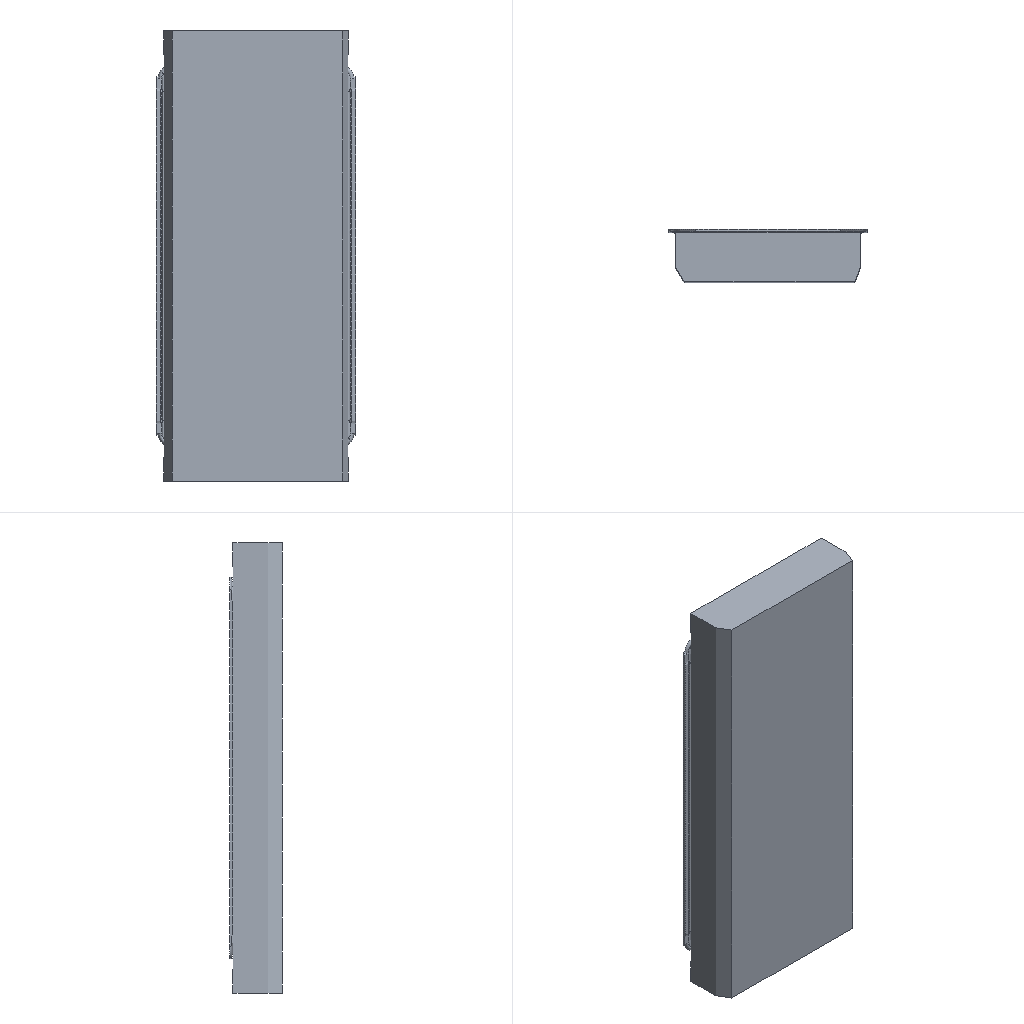Simulation study | ansys workbench
Set-up summary:
category,name,step,type,value,unit,region
solver,ansys_mapdl
solver,version,,,22.1
units,MPA,,stated
analysis,deck,,static,static
load_step,requested,,,1
analysis,nlgeom,,,False
mesh,nodes,,,345798
mesh,elements,,,249801
element_type,ANSYS 187 (type 1),,solid,1742
element_type,ANSYS 187 (type 2),,solid,204561
element_type,ANSYS 174 (type 3),,contact,7261
element_type,ANSYS 170 (type 4),,target,7261
element_type,ANSYS 154 (type 5),,surface,28976
load,load commands in deck,,count,1
bc,support commands in deck,,count,1
named_set,_FIXEDSU,,component
material,1,,in results
material,2,,in results
check,setup vs results,,match,28976 surface effect element(s) are not in the reader's mesh and were not compared
Ansys APDL input file, long lists of numbers shortened:
/batch
/config,noeldb,1     ! force off writing results to database
*get,_wallstrt,active,,time,wall
! ANSYS input file written by Workbench version 2022 R1
! File used for geometry attach: F:\ansys（分析文件汇总)\橡胶有限元分析\装配体简化.x_t
/title,wbnew--____ (B5)
! ****** Begin Custom Load Command Snippet ******
/COM, ACT Extensions:
/COM,     LSDYNA, 2021.1
/COM,
! ****** End   Custom Load Command Snippet ******
*DIM,_wb_ProjectScratch_dir,string,248
_wb_ProjectScratch_dir(1) = 'C:\Users\Administrator\AppData\Local\Temp\WB_Administrator_11288_2\_ProjectScratch\Scr4300\'
*DIM,_wb_SolverFiles_dir,string,248
_wb_SolverFiles_dir(1) = 'C:\Users\Administrator\AppData\Local\Temp\WB_Administrator_11288_2\wbnew_files\dp0\SYS\MECH\'
*DIM,_wb_userfiles_dir,string,248
_wb_userfiles_dir(1) = 'C:\Users\Administrator\AppData\Local\Temp\WB_Administrator_11288_2\wbnew_files\user_files\'
/com,--- Data in consistent NMM units. See Solving Units in the help system for more information.
/units,MPA
/nopr
/wb,file,start              !  signify a WB generated input file
/prep7
! Turn off shape checking because checks already performed inside WB mesher.
! See help system for more information.
SHPP,OFF,,NOWARN
/nolist
etcon,set             ! allow ANSYS to choose best KEYOP's for 180x elements, resets any applicable keyopt to MAPDL defaults
/com,*********** Nodes for the whole assembly ***********
nblock,3,,380377
(1i9,3e20.9e3)
        1    -7.883517716E+02    -5.000000000E+01    -1.894807621E+03
! (345797 more lines like these left out)
-1
/wb,elem,start            !  set before creation of elements
/com,*********** Elements for Body 1 "___" ***********
et,1,187
eblock,19,solid,,1742
(19i9)
        1        1        1        1        0        0        0        0       10        0        1      470      475      471      636     3080     3083     3076     3082
! (3483 more lines like these left out)
-1
/com,*********** Elements for Body 2 "XPN-10-1" ***********
et,2,187
eblock,19,solid,,204561
(19i9)
        2        2        2        2        0        0        0        0       10        0    11987    12398    45519    55205    54521   127298   331745   127303   127301
! (409121 more lines like these left out)
-1
/wb,elem,end               !  done creating elements
/com,*********** Send User Defined Coordinate System(s) ***********
csys,0
toffst,273.15,  ! Temperature offset from absolute zero
/com,*********** Set Reference Temperature ***********
tref,22.
/wb,mat,start              !  starting to send materials
/com,*********** Send Materials ***********
Temperature = 'TEMP' ! Temperature
MP,DENS,1,7.85e-09,	! tonne mm^-3
MP,ALPX,1,1.2e-05,	! C^-1
MP,C,1,434000000,	! mm^2 s^-2 C^-1
MP,KXX,1,60.5,	! tonne mm s^-3 C^-1
MP,RSVX,1,0.00017,	! ohm mm
MP,EX,1,200000,	! tonne s^-2 mm^-1
MP,NUXY,1,0.3,
MP,MURX,1,10000,
Temperature = 'TEMP' ! Temperature
MP,DENS,2,7.85e-09,	! tonne mm^-3
MP,ALPX,2,1.2e-05,	! C^-1
MP,C,2,434000000,	! mm^2 s^-2 C^-1
MP,KXX,2,60.5,	! tonne mm s^-3 C^-1
MP,RSVX,2,0.00017,	! ohm mm
MP,EX,2,200000,	! tonne s^-2 mm^-1
MP,NUXY,2,0.3,
MP,MURX,2,10000,
/wb,mat,end                !  done sending materials
!************************* Model Summary ********************
!___,	不休钢,	matid,	1
!XPN-10-1,	橡胶,	matid,	2
!************************* End Model Summary ********************
! get the diagonal of the bounding box. Needed later for other things
*get,_xmin,node,,mnloc,x
*get,_ymin,node,,mnloc,y
*get,_zmin,node,,mnloc,z
*get,_xmax,node,,mxloc,x
*get,_ymax,node,,mxloc,y
*get,_zmax,node,,mxloc,z
_ASMDIAG=(_xmax-_xmin)*(_xmax-_xmin)+(_ymax-_ymin)*(_ymax-_ymin)+(_zmax-_zmin)*(_zmax-_zmin)
_ASMDIAG=SQRT(_ASMDIAG)
/wb,contact,start          !  starting to send contact
/com,*********** Create Contact "接触区域" ***********
/com,            Real Constant Set For Above Contact Is 4 & 3
*set,tid,4
*set,cid,3
r,tid
r,cid
et,tid,170
et,cid,174
eblock,10,,,412
(15i9)
   285310        4        4        4        0        6        3      349      349      656      660      349      681
! (411 more lines like these left out)
-1
eblock,10,,,412
(15i9)
   285722        3        3        3        0        6        3      349      349      656      660      349      681
! (411 more lines like these left out)
-1
eblock,10,,,6849
(15i9)
   286134        3        4        3        0    10566    14209    17383    17383   110406   142092    17383   110408
! (6848 more lines like these left out)
-1
eblock,10,,,6849
(15i9)
   292983        4        3        4        0    10566    14209    17383    17383   110406   142092    17383   110408
! (6848 more lines like these left out)
-1
keyo,cid,8,2               ! auto create asymmetric contact (from Program Controlled setting)
keyo,cid,10,0              ! adjust contact stiffness each NR iteration (from Program Controlled setting)
keyo,cid,12,5              ! bonded always
keyo,cid,18,1              ! small sliding turned on by application
keyo,cid,2,0               ! augmented Lagrange (from Program Controlled setting)
keyo,cid,4,0               ! on Gauss point (from Program Controlled setting)
keyo,cid,9,1               ! ignore initial gaps/penetration
keyo,cid,7,0               ! No Prediction
rmod,tid,3,10.      ! FKN
rmod,tid,5,0.       ! ICONT
rmod,tid,6,0.       ! PINB
rmod,tid,10,0.      ! CNOF
rmod,tid,12,0.      ! FKT
rmod,tid,36,29      ! WB DSID
rmod,cid,3,10.      ! FKN
rmod,cid,5,0.       ! ICONT
rmod,cid,6,0.       ! PINB
rmod,cid,10,0.      ! CNOF
rmod,cid,12,0.      ! FKT
rmod,cid,36,29      ! WB DSID
nsel,all
esel,all
/wb,contact,end            !  done creating contacts
/golist
/wb,load,start             !  starting to send loads
/com,*********** Fixed Supports ***********
CMBLOCK,_FIXEDSU,NODE,     2892
(8i10)
        52        65        66        67        68        69        70        71
! (361 more lines like these left out)
cmsel,s,_FIXEDSU
d,all,all
nsel,all
/com,*********** Define Pressure Using Surface Effect Elements "__" ***********
et,5,154
eblock,10,,,28976
(15i9)
   299832        5        5        5        0    23749    32864    26871    26871   194333   226056    26871   194328
! (28975 more lines like these left out)
-1
esel,s,type,,5
keyop,5,7,0                ! Use deformed area for application of load
esel,all
esel,all
/gst,on,on
fini
*get,_numnode,node,0,count
*get,_numelem,elem,0,count
*get, _MAXELEMNUM, elem, 0, NUM, MAX
*get, _MAXNODENUM, node, 0, NUM, MAX
*get, _MAXELEMTYPE, etyp, 0, NUM, MAX
*get, _MAXREALCONST, real, 0, NUM, MAX
/go
/wb,load,end               !  done creating loads
/com,--- Number of total nodes = %_numnode%
/com,--- Number of contact elements = 43498
/com,--- Number of spring elements = 0
/com,--- Number of bearing elements = 0
/com,--- Number of solid elements = 206303
/com,--- Number of condensed parts = 0
/com,--- Number of total elements = %_numelem%
*get,_wallbsol,active,,time,wall
/com,****************************************************************************
/com,*************************    SOLUTION       ********************************
/com,****************************************************************************
/solu
antype,0                   ! static analysis
_thickRatio=0.5     ! Ratio of thick parts in the model
eqsl,sparse,,,,,1
cntr,print,1               ! print out contact info and also make no initial contact an error
dmpoption,emat,no             ! Don't combine emat file for DANSYS
dmpoption,esav,no             ! Don't combine esav file for DANSYS
nldiag,cont,iter           ! print out contact info each equilibrium iteration
rescontrol,,none                 ! Do not keep any restart files
/com,****************************************************
/com,******************* SOLVE FOR LS 1 OF 1 ****************
esel,s,type,,5
nsle
sf,all,pres,100.
nsel,all
esel,all
esel,all
/nopr
/gopr
autots,on                   ! User turned on automatic time stepping
nsub,1,10,1,OFF
time,1.
outres,erase
outres,all,none
outres,nsol,all,
outres,rsol,all
outres,eangl,all
outres,etmp,all
outres,veng,all
outres,strs,all,
outres,epel,all,
outres,eppl,all,
outres,cont,all,
! *********** WB SOLVE COMMAND ***********
! check interactive state
*get,ANSINTER_,active,,int
*if,ANSINTER_,ne,0,then
/eof
*endif
solve
/com *************** Write FE CONNECTORS *********
CEWRITE,file,ce,,INTE
/com,****************************************************
/com,*************** FINISHED SOLVE FOR LS 1 *************
*get,_wallasol,active,,time,wall
/nopr
*get,_numnode,node,0,count
*get,_numelem,elem,0,count
*get, _MAXELEMNUM, elem, 0, NUM, MAX
*get, _MAXNODENUM, node, 0, NUM, MAX,,,INTERNAL
*get, _MAXELEMTYPE, etyp, 0, NUM, MAX
*get, _MAXREALCONST, real, 0, NUM, MAX
/gopr
/post1
xmlo,ENCODING,ISO-8859-1
xmlo,parm
/xml,parm,xml
fini
/gopr
*get,_walldone,active,,time,wall
_preptime=(_wallbsol-_wallstrt)*3600
_solvtime=(_wallasol-_wallbsol)*3600
_posttime=(_walldone-_wallasol)*3600
_totaltim=(_walldone-_wallstrt)*3600
*get,_dlbratio,active,0,solu,dlbr
*get,_combtime,active,0,solu,comb
*get,_ssmode,active,0,solu,ssmm
*get,_ndofs,active,0,solu,ndof
*get,_sol_end_time,active,0,set,time
*if,_sol_end_time,eq,1.,then
/fclean				!clean distributed files
*endif
/com,--- Total number of nodes = %_numnode%
/com,--- Total number of elements = %_numelem%
/com,--- Element load balance ratio = %_dlbratio%
/com,--- Time to combine distributed files = %_combtime%
/com,--- Sparse memory mode = %_ssmode%
/com,--- Number of DOF = %_ndofs%
/wb,file,end               ! done with WB generated input
Results summary:
result,analysis,,,static
result,last_loadstep,,,1
result,primary field,,,displacement
result,reaction total,1,FX,0.03588,N
result,reaction total,1,FY,850286496.732,N
result,reaction total,1,FZ,0.06474,N
result,mass,,,26.385,"NMM: mm, ton, N, s, mV, mA, degC"